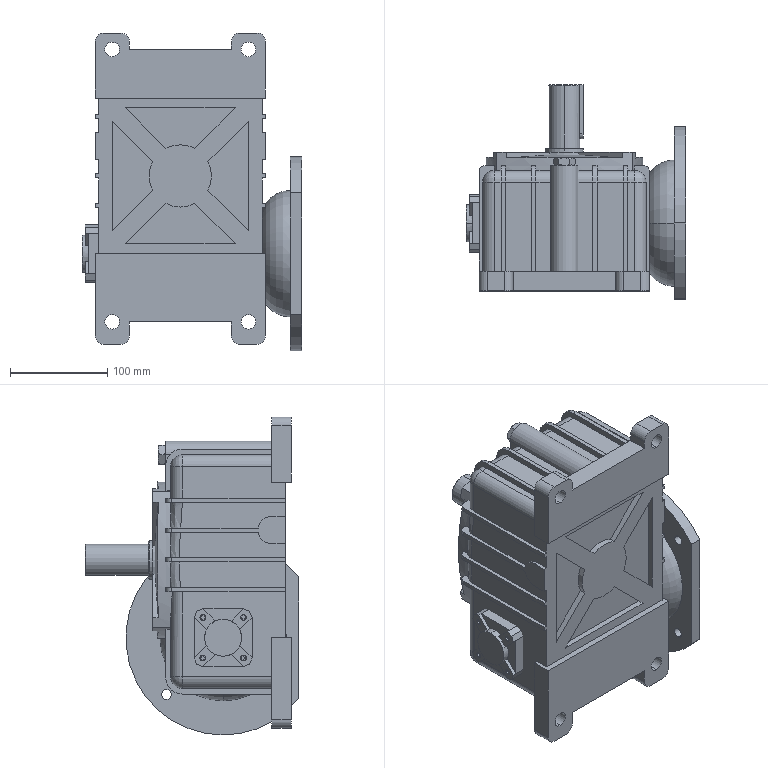Part | SolidWorks | features ICE 30, DeleteBody 8, CirPattern 5, Fillet 5, MirrorSolid 4, LPattern 3, Revolution 3, Chamfer 2, Extrusion 1, MirrorPattern 1, RevCut 1 | 5 solids | 557 faces | box 226 x 220 x 326.9 mm | volume 6279798 mm3 | plane 320 | cylinder 172 | torus 29 | cone 26 | spline 6 | sphere 4 | commonest cylinder face diameters 24 x20 10 x17 26.75 x12 64 x10 34.15 x9 5.653 x8